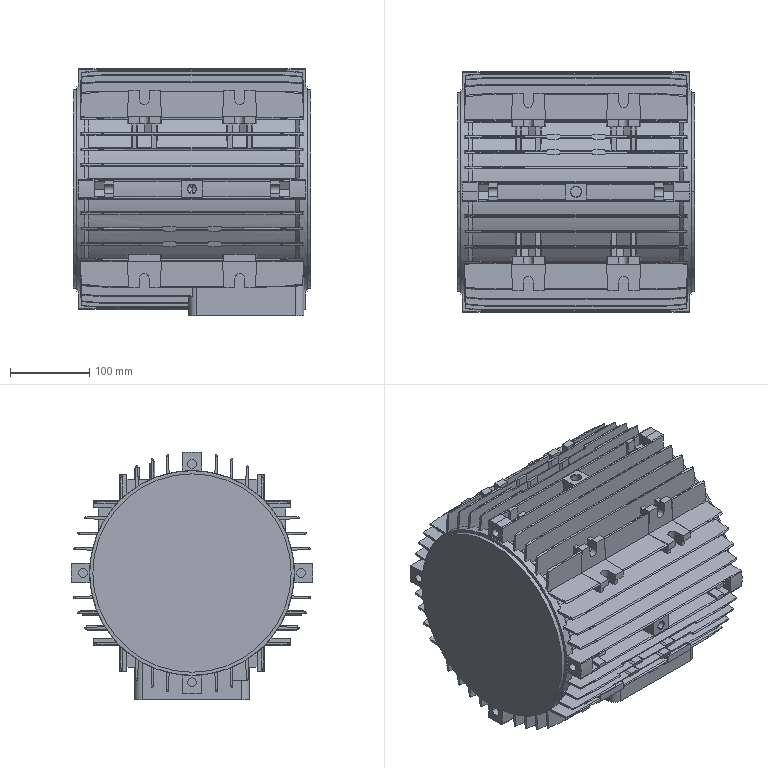Part | STEP file | Input 107 | 1 solid | 1157 faces | box 300 x 305 x 312.5 mm | volume 16733446 mm3 | plane 622 | cylinder 303 | cone 232 | commonest cylinder face diameters 2.4 x102 248 x59 6 x48 11 x24 305 x24 12 x12